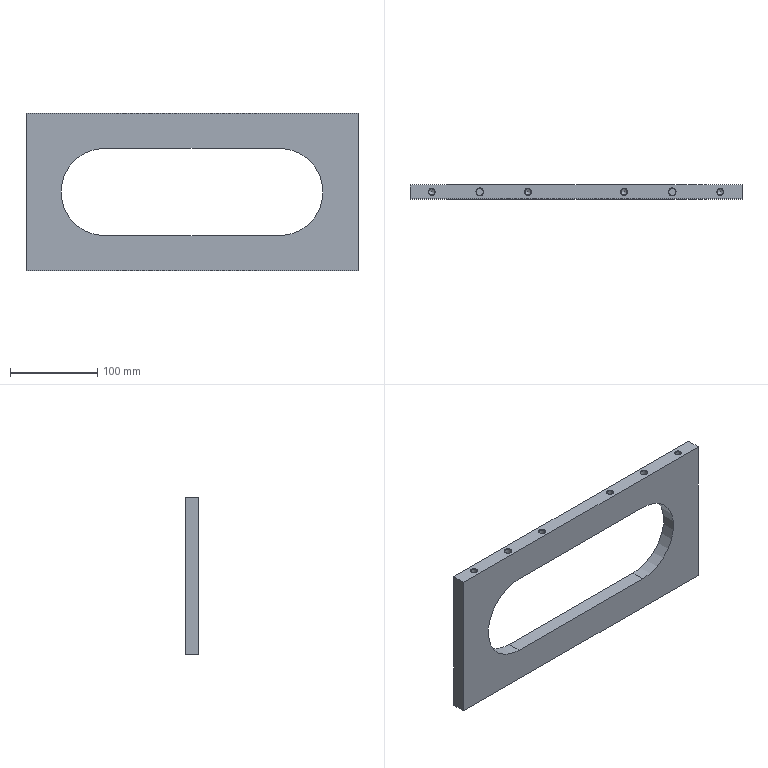Part | STEP file | Tube feed_id1766_x_t | 1 solid | 46 faces | box 380 x 16 x 180 mm | volume 635735 mm3 | cone 20 | cylinder 14 | plane 12 | commonest cylinder face diameters 6.8 x8 8 x4 100 x2